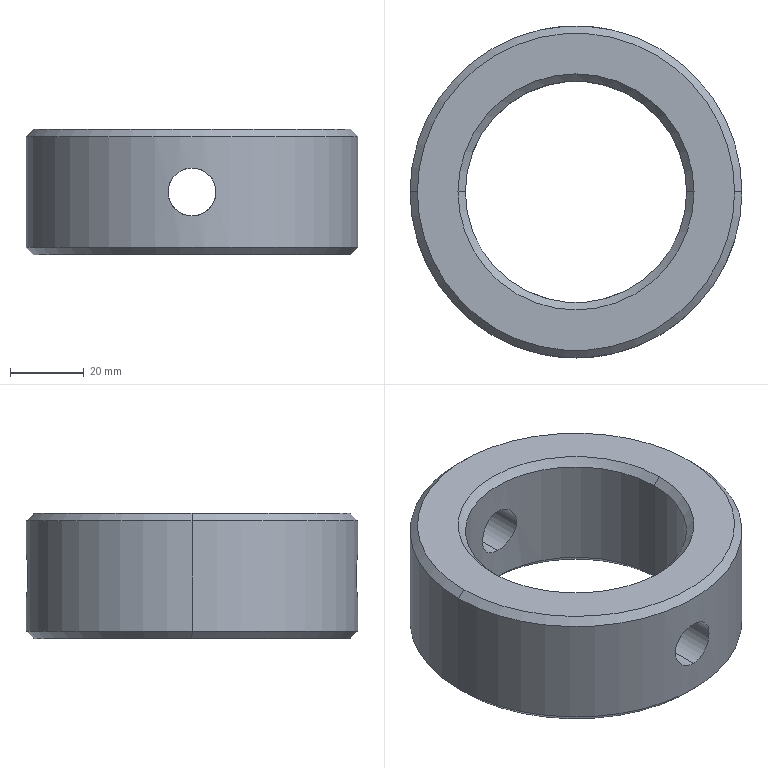Part | SolidWorks | features Chamfer 1, Extrusion 1, ICE 1 | 1 solid | 18 faces | box 90 x 90 x 34 mm | volume 114282 mm3 | cone 8 | cylinder 8 | plane 2 | commonest cylinder face diameters 13 x4 60 x2 90 x2
STEP:
#1=CARTESIAN_POINT('',(43.,0.,34.));
#2=VERTEX_POINT('',#1);
#3=CARTESIAN_POINT('',(-43.,0.,34.));
#4=VERTEX_POINT('',#3);
#5=CARTESIAN_POINT('',(0.,0.,34.));
#6=DIRECTION('',(0.,0.,1.));
#7=DIRECTION('',(1.,0.,0.));
#8=AXIS2_PLACEMENT_3D('',#5,#6,#7);
#9=CIRCLE('',#8,43.);
#10=EDGE_CURVE('',#2,#4,#9,.T.);
#11=ORIENTED_EDGE('',*,*,#10,.F.);
#12=CARTESIAN_POINT('',(45.,0.,32.));
#13=VERTEX_POINT('',#12);
#14=CARTESIAN_POINT('',(43.,0.,34.));
#15=DIRECTION('',(0.7071,0.,-0.7071));
#16=VECTOR('',#15,1000.);
#17=LINE('',#14,#16);
#18=EDGE_CURVE('',#2,#13,#17,.T.);
#19=ORIENTED_EDGE('',*,*,#18,.T.);
#20=CARTESIAN_POINT('',(-45.,0.,32.));
#21=VERTEX_POINT('',#20);
#22=CARTESIAN_POINT('',(0.,0.,32.));
#23=DIRECTION('',(0.,0.,-1.));
#24=DIRECTION('',(1.,0.,0.));
#25=AXIS2_PLACEMENT_3D('',#22,#23,#24);
#26=CIRCLE('',#25,45.);
#27=EDGE_CURVE('',#21,#13,#26,.T.);
#28=ORIENTED_EDGE('',*,*,#27,.F.);
#29=CARTESIAN_POINT('',(-43.,0.,34.));
#30=DIRECTION('',(-0.7071,0.,-0.7071));
#31=VECTOR('',#30,1000.);
#32=LINE('',#29,#31);
#33=EDGE_CURVE('',#4,#21,#32,.T.);
#34=ORIENTED_EDGE('',*,*,#33,.F.);
#35=EDGE_LOOP('',(#11,#19,#28,#34));
#36=FACE_OUTER_BOUND('',#35,.T.);
#37=CARTESIAN_POINT('',(0.,0.,34.));
#38=DIRECTION('',(0.,0.,-1.));
#39=DIRECTION('',(-1.,0.,0.));
#40=AXIS2_PLACEMENT_3D('',#37,#38,#39);
#41=CONICAL_SURFACE('',#40,43.,0.7854);
#42=ADVANCED_FACE('',(#36),#41,.T.);
#43=CARTESIAN_POINT('',(-30.,0.,32.));
#44=VERTEX_POINT('',#43);
#45=CARTESIAN_POINT('',(30.,0.,32.));
#46=VERTEX_POINT('',#45);
#47=CARTESIAN_POINT('',(0.,0.,32.));
#48=DIRECTION('',(0.,0.,1.));
#49=DIRECTION('',(1.,0.,0.));
#50=AXIS2_PLACEMENT_3D('',#47,#48,#49);
#51=CIRCLE('',#50,30.);
#52=EDGE_CURVE('',#44,#46,#51,.T.);
#53=ORIENTED_EDGE('',*,*,#52,.F.);
#54=CARTESIAN_POINT('',(-32.,0.,34.));
#55=VERTEX_POINT('',#54);
#56=CARTESIAN_POINT('',(-30.,0.,32.));
#57=DIRECTION('',(-0.7071,0.,0.7071));
#58=VECTOR('',#57,1000.);
#59=LINE('',#56,#58);
#60=EDGE_CURVE('',#44,#55,#59,.T.);
#61=ORIENTED_EDGE('',*,*,#60,.T.);
#62=CARTESIAN_POINT('',(32.,0.,34.));
#63=VERTEX_POINT('',#62);
#64=CARTESIAN_POINT('',(0.,0.,34.));
#65=DIRECTION('',(0.,0.,-1.));
#66=DIRECTION('',(1.,0.,0.));
#67=AXIS2_PLACEMENT_3D('',#64,#65,#66);
#68=CIRCLE('',#67,32.);
#69=EDGE_CURVE('',#63,#55,#68,.T.);
#70=ORIENTED_EDGE('',*,*,#69,.F.);
#71=CARTESIAN_POINT('',(30.,0.,32.));
#72=DIRECTION('',(0.7071,0.,0.7071));
#73=VECTOR('',#72,1000.);
#74=LINE('',#71,#73);
#75=EDGE_CURVE('',#46,#63,#74,.T.);
#76=ORIENTED_EDGE('',*,*,#75,.F.);
#77=EDGE_LOOP('',(#53,#61,#70,#76));
#78=FACE_OUTER_BOUND('',#77,.T.);
#79=CARTESIAN_POINT('',(0.,0.,32.));
#80=DIRECTION('',(0.,0.,1.));
#81=DIRECTION('',(1.,0.,0.));
#82=AXIS2_PLACEMENT_3D('',#79,#80,#81);
#83=CONICAL_SURFACE('',#82,30.,0.7854);
#84=ADVANCED_FACE('',(#78),#83,.F.);
#85=CARTESIAN_POINT('',(-43.,0.,0.));
#86=VERTEX_POINT('',#85);
#87=CARTESIAN_POINT('',(43.,0.,0.));
#88=VERTEX_POINT('',#87);
#89=CARTESIAN_POINT('',(0.,0.,0.));
#90=DIRECTION('',(0.,0.,-1.));
#91=DIRECTION('',(1.,0.,0.));
#92=AXIS2_PLACEMENT_3D('',#89,#90,#91);
#93=CIRCLE('',#92,43.);
#94=EDGE_CURVE('',#86,#88,#93,.T.);
#95=ORIENTED_EDGE('',*,*,#94,.F.);
#96=CARTESIAN_POINT('',(-45.,0.,2.));
#97=VERTEX_POINT('',#96);
#98=CARTESIAN_POINT('',(-45.,0.,2.));
#99=DIRECTION('',(-0.7071,0.,0.7071));
#100=VECTOR('',#99,1000.);
#101=LINE('',#98,#100);
#102=EDGE_CURVE('',#86,#97,#101,.T.);
#103=ORIENTED_EDGE('',*,*,#102,.T.);
#104=CARTESIAN_POINT('',(45.,0.,2.));
#105=VERTEX_POINT('',#104);
#106=CARTESIAN_POINT('',(0.,0.,2.));
#107=DIRECTION('',(0.,0.,1.));
#108=DIRECTION('',(1.,0.,0.));
#109=AXIS2_PLACEMENT_3D('',#106,#107,#108);
#110=CIRCLE('',#109,45.);
#111=EDGE_CURVE('',#105,#97,#110,.T.);
#112=ORIENTED_EDGE('',*,*,#111,.F.);
#113=CARTESIAN_POINT('',(45.,0.,2.));
#114=DIRECTION('',(0.7071,0.,0.7071));
#115=VECTOR('',#114,1000.);
#116=LINE('',#113,#115);
#117=EDGE_CURVE('',#88,#105,#116,.T.);
#118=ORIENTED_EDGE('',*,*,#117,.F.);
#119=EDGE_LOOP('',(#95,#103,#112,#118));
#120=FACE_OUTER_BOUND('',#119,.T.);
#121=CARTESIAN_POINT('',(0.,0.,2.));
#122=DIRECTION('',(0.,0.,1.));
#123=DIRECTION('',(1.,0.,0.));
#124=AXIS2_PLACEMENT_3D('',#121,#122,#123);
#125=CONICAL_SURFACE('',#124,45.,0.7854);
#126=ADVANCED_FACE('',(#120),#125,.T.);
#127=CARTESIAN_POINT('',(30.,0.,2.));
#128=VERTEX_POINT('',#127);
#129=CARTESIAN_POINT('',(-30.,0.,2.));
#130=VERTEX_POINT('',#129);
#131=CARTESIAN_POINT('',(0.,0.,2.));
#132=DIRECTION('',(0.,0.,-1.));
#133=DIRECTION('',(1.,0.,0.));
#134=AXIS2_PLACEMENT_3D('',#131,#132,#133);
#135=CIRCLE('',#134,30.);
#136=EDGE_CURVE('',#128,#130,#135,.T.);
#137=ORIENTED_EDGE('',*,*,#136,.F.);
#138=CARTESIAN_POINT('',(32.,0.,0.));
#139=VERTEX_POINT('',#138);
#140=CARTESIAN_POINT('',(32.,0.,0.));
#141=DIRECTION('',(0.7071,0.,-0.7071));
#142=VECTOR('',#141,1000.);
#143=LINE('',#140,#142);
#144=EDGE_CURVE('',#128,#139,#143,.T.);
#145=ORIENTED_EDGE('',*,*,#144,.T.);
#146=CARTESIAN_POINT('',(-32.,0.,0.));
#147=VERTEX_POINT('',#146);
#148=CARTESIAN_POINT('',(0.,0.,0.));
#149=DIRECTION('',(0.,0.,1.));
#150=DIRECTION('',(1.,0.,0.));
#151=AXIS2_PLACEMENT_3D('',#148,#149,#150);
#152=CIRCLE('',#151,32.);
#153=EDGE_CURVE('',#147,#139,#152,.T.);
#154=ORIENTED_EDGE('',*,*,#153,.F.);
#155=CARTESIAN_POINT('',(-32.,0.,0.));
#156=DIRECTION('',(-0.7071,0.,-0.7071));
#157=VECTOR('',#156,1000.);
#158=LINE('',#155,#157);
#159=EDGE_CURVE('',#130,#147,#158,.T.);
#160=ORIENTED_EDGE('',*,*,#159,.F.);
#161=EDGE_LOOP('',(#137,#145,#154,#160));
#162=FACE_OUTER_BOUND('',#161,.T.);
#163=CARTESIAN_POINT('',(0.,0.,0.));
#164=DIRECTION('',(0.,0.,-1.));
#165=DIRECTION('',(-1.,0.,0.));
#166=AXIS2_PLACEMENT_3D('',#163,#164,#165);
#167=CONICAL_SURFACE('',#166,32.,0.7854);
#168=ADVANCED_FACE('',(#162),#167,.F.);
#169=CARTESIAN_POINT('',(0.,-45.,10.5));
#170=VERTEX_POINT('',#169);
#171=CARTESIAN_POINT('',(0.,-45.,23.5));
#172=VERTEX_POINT('',#171);
#173=CARTESIAN_POINT('',(0.,-45.,10.5));
#174=CARTESIAN_POINT('',(-0.4244,-45.,10.5));
#175=CARTESIAN_POINT('',(-0.8466,-44.994,10.541));
#176=CARTESIAN_POINT('',(-1.477,-44.976,10.666));
#177=CARTESIAN_POINT('',(-1.685,-44.969,10.719));
#178=CARTESIAN_POINT('',(-2.092,-44.952,10.842));
#179=CARTESIAN_POINT('',(-2.491,-44.932,10.985));
#180=CARTESIAN_POINT('',(-2.875,-44.908,11.166));
#181=CARTESIAN_POINT('',(-3.25,-44.883,11.367));
#182=CARTESIAN_POINT('',(-3.434,-44.869,11.477));
#183=CARTESIAN_POINT('',(-3.967,-44.826,11.833));
#184=CARTESIAN_POINT('',(-4.293,-44.796,12.101));
#185=CARTESIAN_POINT('',(-4.893,-44.734,12.7));
#186=CARTESIAN_POINT('',(-5.167,-44.703,13.034));
#187=CARTESIAN_POINT('',(-5.639,-44.646,13.739));
#188=CARTESIAN_POINT('',(-5.839,-44.62,14.112));
#189=CARTESIAN_POINT('',(-6.084,-44.587,14.702));
#190=CARTESIAN_POINT('',(-6.157,-44.577,14.905));
#191=CARTESIAN_POINT('',(-6.281,-44.56,15.313));
#192=CARTESIAN_POINT('',(-6.333,-44.552,15.519));
#193=CARTESIAN_POINT('',(-6.457,-44.534,16.143));
#194=CARTESIAN_POINT('',(-6.5,-44.528,16.566));
#195=CARTESIAN_POINT('',(-6.5,-44.528,17.425));
#196=CARTESIAN_POINT('',(-6.458,-44.534,17.848));
#197=CARTESIAN_POINT('',(-6.335,-44.552,18.472));
#198=CARTESIAN_POINT('',(-6.283,-44.559,18.678));
#199=CARTESIAN_POINT('',(-6.16,-44.576,19.087));
#200=CARTESIAN_POINT('',(-6.087,-44.586,19.29));
#201=CARTESIAN_POINT('',(-5.843,-44.619,19.88));
#202=CARTESIAN_POINT('',(-5.643,-44.645,20.253));
#203=CARTESIAN_POINT('',(-5.172,-44.702,20.96));
#204=CARTESIAN_POINT('',(-4.898,-44.734,21.294));
#205=CARTESIAN_POINT('',(-4.3,-44.795,21.893));
#206=CARTESIAN_POINT('',(-3.974,-44.826,22.162));
#207=CARTESIAN_POINT('',(-3.263,-44.883,22.638));
#208=CARTESIAN_POINT('',(-2.887,-44.909,22.839));
#209=CARTESIAN_POINT('',(-2.3,-44.942,23.083));
#210=CARTESIAN_POINT('',(-2.101,-44.951,23.155));
#211=CARTESIAN_POINT('',(-1.694,-44.969,23.279));
#212=CARTESIAN_POINT('',(-1.485,-44.976,23.332));
#213=CARTESIAN_POINT('',(-0.8549,-44.994,23.458));
#214=CARTESIAN_POINT('',(-0.43,-45.,23.5));
#215=CARTESIAN_POINT('',(0.,-45.,23.5));
#216=B_SPLINE_CURVE_WITH_KNOTS('',3,(#173,#174,#175,#176,#177,#178,#179,#180,#181,#182,#183,#184,#185,#186,#187,#188,#189,#190,#191,#192,#193,#194,#195,#196,#197,#198,#199,#200,#201,#202,#203,#204,#205,#206,#207,#208,#209,#210,#211,#212,#213,#214,#215),.UNSPECIFIED.,.F.,.F.,(4,2,2,1,2,2,2,2,2,2,2,2,2,2,2,2,2,2,2,2,2,4),(0.02035,0.02162,0.02226,0.02289,0.02353,0.02416,0.02543,0.02671,0.02798,0.02861,0.02925,0.03052,0.03179,0.03243,0.03306,0.03433,0.03561,0.03688,0.03815,0.03878,0.03942,0.04069),.UNSPECIFIED.);
#217=EDGE_CURVE('',#170,#172,#216,.T.);
#218=ORIENTED_EDGE('',*,*,#217,.F.);
#219=CARTESIAN_POINT('',(0.,-30.,10.5));
#220=VERTEX_POINT('',#219);
#221=CARTESIAN_POINT('',(0.,-45.,10.5));
#222=DIRECTION('',(0.,1.,0.));
#223=VECTOR('',#222,1000.);
#224=LINE('',#221,#223);
#225=EDGE_CURVE('',#170,#220,#224,.T.);
#226=ORIENTED_EDGE('',*,*,#225,.T.);
#227=CARTESIAN_POINT('',(0.,-30.,23.5));
#228=VERTEX_POINT('',#227);
#229=CARTESIAN_POINT('',(0.,-30.,10.5));
#230=CARTESIAN_POINT('',(-0.4248,-30.,10.5));
#231=CARTESIAN_POINT('',(-0.848,-29.991,10.541));
#232=CARTESIAN_POINT('',(-1.691,-29.955,10.709));
#233=CARTESIAN_POINT('',(-2.099,-29.929,10.834));
#234=CARTESIAN_POINT('',(-2.686,-29.88,11.077));
#235=CARTESIAN_POINT('',(-2.877,-29.862,11.168));
#236=CARTESIAN_POINT('',(-3.253,-29.824,11.369));
#237=CARTESIAN_POINT('',(-3.438,-29.803,11.479));
#238=CARTESIAN_POINT('',(-3.968,-29.739,11.834));
#239=CARTESIAN_POINT('',(-4.294,-29.693,12.102));
#240=CARTESIAN_POINT('',(-4.894,-29.6,12.701));
#241=CARTESIAN_POINT('',(-5.167,-29.553,13.034));
#242=CARTESIAN_POINT('',(-5.638,-29.466,13.737));
#243=CARTESIAN_POINT('',(-5.838,-29.427,14.11));
#244=CARTESIAN_POINT('',(-6.084,-29.377,14.702));
#245=CARTESIAN_POINT('',(-6.157,-29.362,14.904));
#246=CARTESIAN_POINT('',(-6.281,-29.335,15.312));
#247=CARTESIAN_POINT('',(-6.384,-29.313,15.723));
#248=CARTESIAN_POINT('',(-6.447,-29.299,16.143));
#249=CARTESIAN_POINT('',(-6.489,-29.29,16.567));
#250=CARTESIAN_POINT('',(-6.5,-29.287,16.783));
#251=CARTESIAN_POINT('',(-6.5,-29.287,17.426));
#252=CARTESIAN_POINT('',(-6.458,-29.297,17.849));
#253=CARTESIAN_POINT('',(-6.293,-29.333,18.682));
#254=CARTESIAN_POINT('',(-6.167,-29.36,19.097));
#255=CARTESIAN_POINT('',(-5.842,-29.426,19.882));
#256=CARTESIAN_POINT('',(-5.642,-29.466,20.255));
#257=CARTESIAN_POINT('',(-5.288,-29.531,20.786));
#258=CARTESIAN_POINT('',(-5.16,-29.553,20.959));
#259=CARTESIAN_POINT('',(-4.89,-29.599,21.287));
#260=CARTESIAN_POINT('',(-4.748,-29.622,21.444));
#261=CARTESIAN_POINT('',(-4.301,-29.692,21.892));
#262=CARTESIAN_POINT('',(-3.973,-29.738,22.162));
#263=CARTESIAN_POINT('',(-3.262,-29.824,22.638));
#264=CARTESIAN_POINT('',(-2.889,-29.863,22.838));
#265=CARTESIAN_POINT('',(-2.303,-29.912,23.082));
#266=CARTESIAN_POINT('',(-2.103,-29.927,23.154));
#267=CARTESIAN_POINT('',(-1.694,-29.953,23.279));
#268=CARTESIAN_POINT('',(-1.485,-29.964,23.332));
#269=CARTESIAN_POINT('',(-0.8557,-29.991,23.458));
#270=CARTESIAN_POINT('',(-0.4307,-30.,23.5));
#271=CARTESIAN_POINT('',(0.,-30.,23.5));
#272=B_SPLINE_CURVE_WITH_KNOTS('',3,(#229,#230,#231,#232,#233,#234,#235,#236,#237,#238,#239,#240,#241,#242,#243,#244,#245,#246,#247,#248,#249,#250,#251,#252,#253,#254,#255,#256,#257,#258,#259,#260,#261,#262,#263,#264,#265,#266,#267,#268,#269,#270,#271),.UNSPECIFIED.,.F.,.F.,(4,2,2,2,2,2,2,2,2,1,2,2,2,2,2,2,2,2,2,2,2,4),(0.02038,0.02166,0.02293,0.02357,0.0242,0.02548,0.02675,0.02802,0.02866,0.0293,0.02993,0.03057,0.03184,0.03312,0.03439,0.03503,0.03567,0.03694,0.03821,0.03885,0.03949,0.04076),.UNSPECIFIED.);
#273=EDGE_CURVE('',#220,#228,#272,.T.);
#274=ORIENTED_EDGE('',*,*,#273,.T.);
#275=CARTESIAN_POINT('',(0.,-45.,23.5));
#276=DIRECTION('',(0.,1.,0.));
#277=VECTOR('',#276,1000.);
#278=LINE('',#275,#277);
#279=EDGE_CURVE('',#172,#228,#278,.T.);
#280=ORIENTED_EDGE('',*,*,#279,.F.);
#281=EDGE_LOOP('',(#218,#226,#274,#280));
#282=FACE_OUTER_BOUND('',#281,.T.);
#283=CARTESIAN_POINT('',(0.,-45.,17.));
#284=DIRECTION('',(0.,1.,0.));
#285=DIRECTION('',(0.,0.,1.));
#286=AXIS2_PLACEMENT_3D('',#283,#284,#285);
#287=CYLINDRICAL_SURFACE('',#286,6.5);
#288=ADVANCED_FACE('',(#282),#287,.F.);
#289=CARTESIAN_POINT('',(0.,30.,23.5));
#290=VERTEX_POINT('',#289);
#291=CARTESIAN_POINT('',(0.,30.,10.5));
#292=VERTEX_POINT('',#291);
#293=CARTESIAN_POINT('',(0.,30.,23.5));
#294=CARTESIAN_POINT('',(-0.4308,30.,23.5));
#295=CARTESIAN_POINT('',(-0.8542,29.991,23.458));
#296=CARTESIAN_POINT('',(-1.479,29.964,23.333));
#297=CARTESIAN_POINT('',(-1.685,29.953,23.281));
#298=CARTESIAN_POINT('',(-2.094,29.928,23.157));
#299=CARTESIAN_POINT('',(-2.297,29.913,23.084));
#300=CARTESIAN_POINT('',(-2.887,29.863,22.839));
#301=CARTESIAN_POINT('',(-3.26,29.824,22.639));
#302=CARTESIAN_POINT('',(-3.966,29.739,22.168));
#303=CARTESIAN_POINT('',(-4.299,29.692,21.894));
#304=CARTESIAN_POINT('',(-4.896,29.599,21.296));
#305=CARTESIAN_POINT('',(-5.165,29.553,20.97));
#306=CARTESIAN_POINT('',(-5.64,29.466,20.259));
#307=CARTESIAN_POINT('',(-5.841,29.426,19.883));
#308=CARTESIAN_POINT('',(-6.084,29.377,19.297));
#309=CARTESIAN_POINT('',(-6.156,29.362,19.097));
#310=CARTESIAN_POINT('',(-6.28,29.335,18.69));
#311=CARTESIAN_POINT('',(-6.333,29.324,18.48));
#312=CARTESIAN_POINT('',(-6.458,29.297,17.851));
#313=CARTESIAN_POINT('',(-6.5,29.287,17.428));
#314=CARTESIAN_POINT('',(-6.5,29.287,16.577));
#315=CARTESIAN_POINT('',(-6.458,29.297,16.145));
#316=CARTESIAN_POINT('',(-6.291,29.333,15.31));
#317=CARTESIAN_POINT('',(-6.168,29.36,14.905));
#318=CARTESIAN_POINT('',(-5.923,29.41,14.313));
#319=CARTESIAN_POINT('',(-5.83,29.428,14.118));
#320=CARTESIAN_POINT('',(-5.629,29.467,13.743));
#321=CARTESIAN_POINT('',(-5.52,29.488,13.562));
#322=CARTESIAN_POINT('',(-5.168,29.553,13.035));
#323=CARTESIAN_POINT('',(-4.897,29.599,12.705));
#324=CARTESIAN_POINT('',(-4.294,29.693,12.101));
#325=CARTESIAN_POINT('',(-3.967,29.739,11.834));
#326=CARTESIAN_POINT('',(-3.44,29.803,11.481));
#327=CARTESIAN_POINT('',(-3.258,29.823,11.371));
#328=CARTESIAN_POINT('',(-2.881,29.862,11.169));
#329=CARTESIAN_POINT('',(-2.687,29.88,11.077));
#330=CARTESIAN_POINT('',(-2.098,29.929,10.833));
#331=CARTESIAN_POINT('',(-1.692,29.955,10.71));
#332=CARTESIAN_POINT('',(-1.065,29.982,10.584));
#333=CARTESIAN_POINT('',(-0.852,29.989,10.553));
#334=CARTESIAN_POINT('',(-0.4254,29.998,10.51));
#335=CARTESIAN_POINT('',(-0.2125,30.,10.5));
#336=CARTESIAN_POINT('',(0.,30.,10.5));
#337=B_SPLINE_CURVE_WITH_KNOTS('',3,(#293,#294,#295,#296,#297,#298,#299,#300,#301,#302,#303,#304,#305,#306,#307,#308,#309,#310,#311,#312,#313,#314,#315,#316,#317,#318,#319,#320,#321,#322,#323,#324,#325,#326,#327,#328,#329,#330,#331,#332,#333,#334,#335,#336),.UNSPECIFIED.,.F.,.F.,(4,2,2,2,2,2,2,2,2,2,2,2,2,2,2,2,2,2,2,2,2,4),(0.,0.001274,0.001911,0.002548,0.003822,0.005096,0.00637,0.007643,0.00828,0.008917,0.01019,0.01147,0.01274,0.01338,0.01401,0.01529,0.01656,0.0172,0.01783,0.01911,0.01975,0.02038),.UNSPECIFIED.);
#338=EDGE_CURVE('',#290,#292,#337,.T.);
#339=ORIENTED_EDGE('',*,*,#338,.T.);
#340=CARTESIAN_POINT('',(0.,45.,10.5));
#341=VERTEX_POINT('',#340);
#342=CARTESIAN_POINT('',(0.,-45.,10.5));
#343=DIRECTION('',(0.,1.,0.));
#344=VECTOR('',#343,1000.);
#345=LINE('',#342,#344);
#346=EDGE_CURVE('',#292,#341,#345,.T.);
#347=ORIENTED_EDGE('',*,*,#346,.T.);
#348=CARTESIAN_POINT('',(0.,45.,23.5));
#349=VERTEX_POINT('',#348);
#350=CARTESIAN_POINT('',(0.,45.,23.5));
#351=CARTESIAN_POINT('',(-0.4301,45.,23.5));
#352=CARTESIAN_POINT('',(-0.8529,44.994,23.458));
#353=CARTESIAN_POINT('',(-1.477,44.976,23.334));
#354=CARTESIAN_POINT('',(-1.683,44.969,23.282));
#355=CARTESIAN_POINT('',(-2.091,44.952,23.158));
#356=CARTESIAN_POINT('',(-2.294,44.942,23.085));
#357=CARTESIAN_POINT('',(-2.885,44.909,22.84));
#358=CARTESIAN_POINT('',(-3.258,44.883,22.641));
#359=CARTESIAN_POINT('',(-3.964,44.826,22.169));
#360=CARTESIAN_POINT('',(-4.298,44.795,21.895));
#361=CARTESIAN_POINT('',(-4.897,44.734,21.296));
#362=CARTESIAN_POINT('',(-5.165,44.703,20.969));
#363=CARTESIAN_POINT('',(-5.522,44.66,20.436));
#364=CARTESIAN_POINT('',(-5.632,44.646,20.252));
#365=CARTESIAN_POINT('',(-5.833,44.621,19.877));
#366=CARTESIAN_POINT('',(-6.014,44.597,19.494));
#367=CARTESIAN_POINT('',(-6.157,44.577,19.095));
#368=CARTESIAN_POINT('',(-6.281,44.56,18.688));
#369=CARTESIAN_POINT('',(-6.333,44.552,18.479));
#370=CARTESIAN_POINT('',(-6.458,44.534,17.849));
#371=CARTESIAN_POINT('',(-6.5,44.528,17.427));
#372=CARTESIAN_POINT('',(-6.5,44.528,16.578));
#373=CARTESIAN_POINT('',(-6.458,44.534,16.147));
#374=CARTESIAN_POINT('',(-6.291,44.558,15.312));
#375=CARTESIAN_POINT('',(-6.169,44.576,14.907));
#376=CARTESIAN_POINT('',(-5.924,44.608,14.316));
#377=CARTESIAN_POINT('',(-5.832,44.621,14.121));
#378=CARTESIAN_POINT('',(-5.631,44.646,13.745));
#379=CARTESIAN_POINT('',(-5.521,44.66,13.564));
#380=CARTESIAN_POINT('',(-5.169,44.703,13.036));
#381=CARTESIAN_POINT('',(-4.899,44.734,12.707));
#382=CARTESIAN_POINT('',(-4.294,44.796,12.101));
#383=CARTESIAN_POINT('',(-3.966,44.826,11.833));
#384=CARTESIAN_POINT('',(-3.438,44.869,11.48));
#385=CARTESIAN_POINT('',(-3.256,44.882,11.37));
#386=CARTESIAN_POINT('',(-2.88,44.908,11.169));
#387=CARTESIAN_POINT('',(-2.685,44.92,11.077));
#388=CARTESIAN_POINT('',(-2.095,44.953,10.832));
#389=CARTESIAN_POINT('',(-1.69,44.97,10.709));
#390=CARTESIAN_POINT('',(-0.8557,44.994,10.543));
#391=CARTESIAN_POINT('',(-0.4245,45.,10.5));
#392=CARTESIAN_POINT('',(0.,45.,10.5));
#393=B_SPLINE_CURVE_WITH_KNOTS('',3,(#350,#351,#352,#353,#354,#355,#356,#357,#358,#359,#360,#361,#362,#363,#364,#365,#366,#367,#368,#369,#370,#371,#372,#373,#374,#375,#376,#377,#378,#379,#380,#381,#382,#383,#384,#385,#386,#387,#388,#389,#390,#391,#392),.UNSPECIFIED.,.F.,.F.,(4,2,2,2,2,2,2,2,1,2,2,2,2,2,2,2,2,2,2,2,2,4),(0.,0.001272,0.001908,0.002544,0.003815,0.005087,0.006359,0.006995,0.007631,0.008267,0.008903,0.01017,0.01145,0.01272,0.01335,0.01399,0.01526,0.01653,0.01717,0.01781,0.01908,0.02035),.UNSPECIFIED.);
#394=EDGE_CURVE('',#349,#341,#393,.T.);
#395=ORIENTED_EDGE('',*,*,#394,.F.);
#396=CARTESIAN_POINT('',(0.,-45.,23.5));
#397=DIRECTION('',(0.,1.,0.));
#398=VECTOR('',#397,1000.);
#399=LINE('',#396,#398);
#400=EDGE_CURVE('',#290,#349,#399,.T.);
#401=ORIENTED_EDGE('',*,*,#400,.F.);
#402=EDGE_LOOP('',(#339,#347,#395,#401));
#403=FACE_OUTER_BOUND('',#402,.T.);
#404=CARTESIAN_POINT('',(0.,-45.,17.));
#405=DIRECTION('',(0.,1.,0.));
#406=DIRECTION('',(0.,0.,1.));
#407=AXIS2_PLACEMENT_3D('',#404,#405,#406);
#408=CYLINDRICAL_SURFACE('',#407,6.5);
#409=ADVANCED_FACE('',(#403),#408,.F.);
#410=CARTESIAN_POINT('',(0.,-30.,23.5));
#411=CARTESIAN_POINT('',(0.4308,-30.,23.5));
#412=CARTESIAN_POINT('',(0.8542,-29.991,23.458));
#413=CARTESIAN_POINT('',(1.479,-29.964,23.333));
#414=CARTESIAN_POINT('',(1.685,-29.953,23.281));
#415=CARTESIAN_POINT('',(2.094,-29.928,23.157));
#416=CARTESIAN_POINT('',(2.297,-29.913,23.084));
#417=CARTESIAN_POINT('',(2.887,-29.863,22.839));
#418=CARTESIAN_POINT('',(3.26,-29.824,22.639));
#419=CARTESIAN_POINT('',(3.966,-29.739,22.168));
#420=CARTESIAN_POINT('',(4.299,-29.692,21.894));
#421=CARTESIAN_POINT('',(4.896,-29.599,21.296));
#422=CARTESIAN_POINT('',(5.165,-29.553,20.97));
#423=CARTESIAN_POINT('',(5.64,-29.466,20.259));
#424=CARTESIAN_POINT('',(5.841,-29.426,19.883));
#425=CARTESIAN_POINT('',(6.084,-29.377,19.297));
#426=CARTESIAN_POINT('',(6.156,-29.362,19.097));
#427=CARTESIAN_POINT('',(6.28,-29.335,18.69));
#428=CARTESIAN_POINT('',(6.333,-29.324,18.48));
#429=CARTESIAN_POINT('',(6.458,-29.297,17.851));
#430=CARTESIAN_POINT('',(6.5,-29.287,17.428));
#431=CARTESIAN_POINT('',(6.5,-29.287,16.577));
#432=CARTESIAN_POINT('',(6.458,-29.297,16.145));
#433=CARTESIAN_POINT('',(6.291,-29.333,15.31));
#434=CARTESIAN_POINT('',(6.168,-29.36,14.905));
#435=CARTESIAN_POINT('',(5.923,-29.41,14.313));
#436=CARTESIAN_POINT('',(5.83,-29.428,14.118));
#437=CARTESIAN_POINT('',(5.629,-29.467,13.743));
#438=CARTESIAN_POINT('',(5.52,-29.488,13.562));
#439=CARTESIAN_POINT('',(5.168,-29.553,13.035));
#440=CARTESIAN_POINT('',(4.897,-29.599,12.705));
#441=CARTESIAN_POINT('',(4.294,-29.693,12.101));
#442=CARTESIAN_POINT('',(3.967,-29.739,11.834));
#443=CARTESIAN_POINT('',(3.44,-29.803,11.481));
#444=CARTESIAN_POINT('',(3.258,-29.823,11.371));
#445=CARTESIAN_POINT('',(2.881,-29.862,11.169));
#446=CARTESIAN_POINT('',(2.687,-29.88,11.077));
#447=CARTESIAN_POINT('',(2.098,-29.929,10.833));
#448=CARTESIAN_POINT('',(1.692,-29.955,10.71));
#449=CARTESIAN_POINT('',(1.065,-29.982,10.584));
#450=CARTESIAN_POINT('',(0.852,-29.989,10.553));
#451=CARTESIAN_POINT('',(0.4254,-29.998,10.51));
#452=CARTESIAN_POINT('',(0.2125,-30.,10.5));
#453=CARTESIAN_POINT('',(0.,-30.,10.5));
#454=B_SPLINE_CURVE_WITH_KNOTS('',3,(#410,#411,#412,#413,#414,#415,#416,#417,#418,#419,#420,#421,#422,#423,#424,#425,#426,#427,#428,#429,#430,#431,#432,#433,#434,#435,#436,#437,#438,#439,#440,#441,#442,#443,#444,#445,#446,#447,#448,#449,#450,#451,#452,#453),.UNSPECIFIED.,.F.,.F.,(4,2,2,2,2,2,2,2,2,2,2,2,2,2,2,2,2,2,2,2,2,4),(0.,0.001274,0.001911,0.002548,0.003822,0.005096,0.00637,0.007643,0.00828,0.008917,0.01019,0.01147,0.01274,0.01338,0.01401,0.01529,0.01656,0.0172,0.01783,0.01911,0.01975,0.02038),.UNSPECIFIED.);
#455=EDGE_CURVE('',#228,#220,#454,.T.);
#456=ORIENTED_EDGE('',*,*,#455,.F.);
#457=ORIENTED_EDGE('',*,*,#273,.F.);
#458=EDGE_LOOP('',(#456,#457));
#459=FACE_BOUND('',#458,.T.);
#460=ORIENTED_EDGE('',*,*,#52,.T.);
#461=CARTESIAN_POINT('',(30.,0.,34.));
#462=DIRECTION('',(0.,0.,-1.));
#463=VECTOR('',#462,1000.);
#464=LINE('',#461,#463);
#465=EDGE_CURVE('',#46,#128,#464,.T.);
#466=ORIENTED_EDGE('',*,*,#465,.T.);
#467=ORIENTED_EDGE('',*,*,#136,.T.);
#468=CARTESIAN_POINT('',(-30.,0.,34.));
#469=DIRECTION('',(0.,0.,-1.));
#470=VECTOR('',#469,1000.);
#471=LINE('',#468,#470);
#472=EDGE_CURVE('',#44,#130,#471,.T.);
#473=ORIENTED_EDGE('',*,*,#472,.F.);
#474=EDGE_LOOP('',(#460,#466,#467,#473));
#475=FACE_OUTER_BOUND('',#474,.T.);
#476=CARTESIAN_POINT('',(0.,0.,34.));
#477=DIRECTION('',(0.,0.,-1.));
#478=DIRECTION('',(-1.,0.,0.));
#479=AXIS2_PLACEMENT_3D('',#476,#477,#478);
#480=CYLINDRICAL_SURFACE('',#479,30.);
#481=ADVANCED_FACE('',(#459,#475),#480,.F.);
#482=ORIENTED_EDGE('',*,*,#394,.T.);
#483=CARTESIAN_POINT('',(0.,45.,10.5));
#484=CARTESIAN_POINT('',(0.4244,45.,10.5));
#485=CARTESIAN_POINT('',(0.8466,44.994,10.541));
#486=CARTESIAN_POINT('',(1.477,44.976,10.666));
#487=CARTESIAN_POINT('',(1.685,44.969,10.719));
#488=CARTESIAN_POINT('',(2.092,44.952,10.842));
#489=CARTESIAN_POINT('',(2.491,44.932,10.985));
#490=CARTESIAN_POINT('',(2.875,44.908,11.166));
#491=CARTESIAN_POINT('',(3.25,44.883,11.367));
#492=CARTESIAN_POINT('',(3.434,44.869,11.477));
#493=CARTESIAN_POINT('',(3.967,44.826,11.833));
#494=CARTESIAN_POINT('',(4.293,44.796,12.101));
#495=CARTESIAN_POINT('',(4.893,44.734,12.7));
#496=CARTESIAN_POINT('',(5.167,44.703,13.034));
#497=CARTESIAN_POINT('',(5.639,44.646,13.739));
#498=CARTESIAN_POINT('',(5.839,44.62,14.112));
#499=CARTESIAN_POINT('',(6.084,44.587,14.702));
#500=CARTESIAN_POINT('',(6.157,44.577,14.905));
#501=CARTESIAN_POINT('',(6.281,44.56,15.313));
#502=CARTESIAN_POINT('',(6.333,44.552,15.519));
#503=CARTESIAN_POINT('',(6.457,44.534,16.143));
#504=CARTESIAN_POINT('',(6.5,44.528,16.566));
#505=CARTESIAN_POINT('',(6.5,44.528,17.425));
#506=CARTESIAN_POINT('',(6.458,44.534,17.848));
#507=CARTESIAN_POINT('',(6.335,44.552,18.472));
#508=CARTESIAN_POINT('',(6.283,44.559,18.678));
#509=CARTESIAN_POINT('',(6.16,44.576,19.087));
#510=CARTESIAN_POINT('',(6.087,44.586,19.29));
#511=CARTESIAN_POINT('',(5.843,44.619,19.88));
#512=CARTESIAN_POINT('',(5.643,44.645,20.253));
#513=CARTESIAN_POINT('',(5.172,44.702,20.96));
#514=CARTESIAN_POINT('',(4.898,44.734,21.294));
#515=CARTESIAN_POINT('',(4.3,44.795,21.893));
#516=CARTESIAN_POINT('',(3.974,44.826,22.162));
#517=CARTESIAN_POINT('',(3.263,44.883,22.638));
#518=CARTESIAN_POINT('',(2.887,44.909,22.839));
#519=CARTESIAN_POINT('',(2.3,44.942,23.083));
#520=CARTESIAN_POINT('',(2.101,44.951,23.155));
#521=CARTESIAN_POINT('',(1.694,44.969,23.279));
#522=CARTESIAN_POINT('',(1.485,44.976,23.332));
#523=CARTESIAN_POINT('',(0.8549,44.994,23.458));
#524=CARTESIAN_POINT('',(0.43,45.,23.5));
#525=CARTESIAN_POINT('',(0.,45.,23.5));
#526=B_SPLINE_CURVE_WITH_KNOTS('',3,(#483,#484,#485,#486,#487,#488,#489,#490,#491,#492,#493,#494,#495,#496,#497,#498,#499,#500,#501,#502,#503,#504,#505,#506,#507,#508,#509,#510,#511,#512,#513,#514,#515,#516,#517,#518,#519,#520,#521,#522,#523,#524,#525),.UNSPECIFIED.,.F.,.F.,(4,2,2,1,2,2,2,2,2,2,2,2,2,2,2,2,2,2,2,2,2,4),(0.02035,0.02162,0.02226,0.02289,0.02353,0.02416,0.02543,0.02671,0.02798,0.02861,0.02925,0.03052,0.03179,0.03243,0.03306,0.03433,0.03561,0.03688,0.03815,0.03878,0.03942,0.04069),.UNSPECIFIED.);
#527=EDGE_CURVE('',#341,#349,#526,.T.);
#528=ORIENTED_EDGE('',*,*,#527,.T.);
#529=EDGE_LOOP('',(#482,#528));
#530=FACE_BOUND('',#529,.T.);
#531=ORIENTED_EDGE('',*,*,#27,.T.);
#532=CARTESIAN_POINT('',(45.,0.,34.));
#533=DIRECTION('',(0.,0.,-1.));
#534=VECTOR('',#533,1000.);
#535=LINE('',#532,#534);
#536=EDGE_CURVE('',#13,#105,#535,.T.);
#537=ORIENTED_EDGE('',*,*,#536,.T.);
#538=ORIENTED_EDGE('',*,*,#111,.T.);
#539=CARTESIAN_POINT('',(-45.,0.,34.));
#540=DIRECTION('',(0.,0.,-1.));
#541=VECTOR('',#540,1000.);
#542=LINE('',#539,#541);
#543=EDGE_CURVE('',#21,#97,#542,.T.);
#544=ORIENTED_EDGE('',*,*,#543,.F.);
#545=EDGE_LOOP('',(#531,#537,#538,#544));
#546=FACE_OUTER_BOUND('',#545,.T.);
#547=CARTESIAN_POINT('',(0.,0.,34.));
#548=DIRECTION('',(0.,0.,-1.));
#549=DIRECTION('',(-1.,0.,0.));
#550=AXIS2_PLACEMENT_3D('',#547,#548,#549);
#551=CYLINDRICAL_SURFACE('',#550,45.);
#552=ADVANCED_FACE('',(#530,#546),#551,.T.);
#553=ORIENTED_EDGE('',*,*,#69,.T.);
#554=CARTESIAN_POINT('',(0.,0.,34.));
#555=DIRECTION('',(0.,0.,-1.));
#556=DIRECTION('',(1.,0.,0.));
#557=AXIS2_PLACEMENT_3D('',#554,#555,#556);
#558=CIRCLE('',#557,32.);
#559=EDGE_CURVE('',#55,#63,#558,.T.);
#560=ORIENTED_EDGE('',*,*,#559,.T.);
#561=EDGE_LOOP('',(#553,#560));
#562=FACE_BOUND('',#561,.T.);
#563=CARTESIAN_POINT('',(0.,0.,34.));
#564=DIRECTION('',(0.,0.,1.));
#565=DIRECTION('',(1.,0.,0.));
#566=AXIS2_PLACEMENT_3D('',#563,#564,#565);
#567=CIRCLE('',#566,43.);
#568=EDGE_CURVE('',#4,#2,#567,.T.);
#569=ORIENTED_EDGE('',*,*,#568,.T.);
#570=ORIENTED_EDGE('',*,*,#10,.T.);
#571=EDGE_LOOP('',(#569,#570));
#572=FACE_OUTER_BOUND('',#571,.T.);
#573=CARTESIAN_POINT('',(0.,0.,34.));
#574=DIRECTION('',(0.,0.,1.));
#575=DIRECTION('',(1.,0.,0.));
#576=AXIS2_PLACEMENT_3D('',#573,#574,#575);
#577=PLANE('',#576);
#578=ADVANCED_FACE('',(#562,#572),#577,.T.);
#579=ORIENTED_EDGE('',*,*,#153,.T.);
#580=CARTESIAN_POINT('',(0.,0.,0.));
#581=DIRECTION('',(0.,0.,1.));
#582=DIRECTION('',(1.,0.,0.));
#583=AXIS2_PLACEMENT_3D('',#580,#581,#582);
#584=CIRCLE('',#583,32.);
#585=EDGE_CURVE('',#139,#147,#584,.T.);
#586=ORIENTED_EDGE('',*,*,#585,.T.);
#587=EDGE_LOOP('',(#579,#586));
#588=FACE_BOUND('',#587,.T.);
#589=CARTESIAN_POINT('',(0.,0.,0.));
#590=DIRECTION('',(0.,0.,-1.));
#591=DIRECTION('',(1.,0.,0.));
#592=AXIS2_PLACEMENT_3D('',#589,#590,#591);
#593=CIRCLE('',#592,43.);
#594=EDGE_CURVE('',#88,#86,#593,.T.);
#595=ORIENTED_EDGE('',*,*,#594,.T.);
#596=ORIENTED_EDGE('',*,*,#94,.T.);
#597=EDGE_LOOP('',(#595,#596));
#598=FACE_OUTER_BOUND('',#597,.T.);
#599=CARTESIAN_POINT('',(0.,0.,0.));
#600=DIRECTION('',(0.,0.,1.));
#601=DIRECTION('',(1.,0.,0.));
#602=AXIS2_PLACEMENT_3D('',#599,#600,#601);
#603=PLANE('',#602);
#604=ADVANCED_FACE('',(#588,#598),#603,.F.);
#605=ORIENTED_EDGE('',*,*,#536,.F.);
#606=CARTESIAN_POINT('',(0.,0.,32.));
#607=DIRECTION('',(0.,0.,-1.));
#608=DIRECTION('',(1.,0.,0.));
#609=AXIS2_PLACEMENT_3D('',#606,#607,#608);
#610=CIRCLE('',#609,45.);
#611=EDGE_CURVE('',#13,#21,#610,.T.);
#612=ORIENTED_EDGE('',*,*,#611,.T.);
#613=ORIENTED_EDGE('',*,*,#543,.T.);
#614=CARTESIAN_POINT('',(0.,0.,2.));
#615=DIRECTION('',(0.,0.,1.));
#616=DIRECTION('',(1.,0.,0.));
#617=AXIS2_PLACEMENT_3D('',#614,#615,#616);
#618=CIRCLE('',#617,45.);
#619=EDGE_CURVE('',#97,#105,#618,.T.);
#620=ORIENTED_EDGE('',*,*,#619,.T.);
#621=EDGE_LOOP('',(#605,#612,#613,#620));
#622=FACE_OUTER_BOUND('',#621,.T.);
#623=CARTESIAN_POINT('',(0.,-45.,23.5));
#624=CARTESIAN_POINT('',(0.4301,-45.,23.5));
#625=CARTESIAN_POINT('',(0.8529,-44.994,23.458));
#626=CARTESIAN_POINT('',(1.477,-44.976,23.334));
#627=CARTESIAN_POINT('',(1.683,-44.969,23.282));
#628=CARTESIAN_POINT('',(2.091,-44.952,23.158));
#629=CARTESIAN_POINT('',(2.294,-44.942,23.085));
#630=CARTESIAN_POINT('',(2.885,-44.909,22.84));
#631=CARTESIAN_POINT('',(3.258,-44.883,22.641));
#632=CARTESIAN_POINT('',(3.964,-44.826,22.169));
#633=CARTESIAN_POINT('',(4.298,-44.795,21.895));
#634=CARTESIAN_POINT('',(4.897,-44.734,21.296));
#635=CARTESIAN_POINT('',(5.165,-44.703,20.969));
#636=CARTESIAN_POINT('',(5.522,-44.66,20.436));
#637=CARTESIAN_POINT('',(5.632,-44.646,20.252));
#638=CARTESIAN_POINT('',(5.833,-44.621,19.877));
#639=CARTESIAN_POINT('',(6.014,-44.597,19.494));
#640=CARTESIAN_POINT('',(6.157,-44.577,19.095));
#641=CARTESIAN_POINT('',(6.281,-44.56,18.688));
#642=CARTESIAN_POINT('',(6.333,-44.552,18.479));
#643=CARTESIAN_POINT('',(6.458,-44.534,17.849));
#644=CARTESIAN_POINT('',(6.5,-44.528,17.427));
#645=CARTESIAN_POINT('',(6.5,-44.528,16.578));
#646=CARTESIAN_POINT('',(6.458,-44.534,16.147));
#647=CARTESIAN_POINT('',(6.291,-44.558,15.312));
#648=CARTESIAN_POINT('',(6.169,-44.576,14.907));
#649=CARTESIAN_POINT('',(5.924,-44.608,14.316));
#650=CARTESIAN_POINT('',(5.832,-44.621,14.121));
#651=CARTESIAN_POINT('',(5.631,-44.646,13.745));
#652=CARTESIAN_POINT('',(5.521,-44.66,13.564));
#653=CARTESIAN_POINT('',(5.169,-44.703,13.036));
#654=CARTESIAN_POINT('',(4.899,-44.734,12.707));
#655=CARTESIAN_POINT('',(4.294,-44.796,12.101));
#656=CARTESIAN_POINT('',(3.966,-44.826,11.833));
#657=CARTESIAN_POINT('',(3.438,-44.869,11.48));
#658=CARTESIAN_POINT('',(3.256,-44.882,11.37));
#659=CARTESIAN_POINT('',(2.88,-44.908,11.169));
#660=CARTESIAN_POINT('',(2.685,-44.92,11.077));
#661=CARTESIAN_POINT('',(2.095,-44.953,10.832));
#662=CARTESIAN_POINT('',(1.69,-44.97,10.709));
#663=CARTESIAN_POINT('',(0.8557,-44.994,10.543));
#664=CARTESIAN_POINT('',(0.4245,-45.,10.5));
#665=CARTESIAN_POINT('',(0.,-45.,10.5));
#666=B_SPLINE_CURVE_WITH_KNOTS('',3,(#623,#624,#625,#626,#627,#628,#629,#630,#631,#632,#633,#634,#635,#636,#637,#638,#639,#640,#641,#642,#643,#644,#645,#646,#647,#648,#649,#650,#651,#652,#653,#654,#655,#656,#657,#658,#659,#660,#661,#662,#663,#664,#665),.UNSPECIFIED.,.F.,.F.,(4,2,2,2,2,2,2,2,1,2,2,2,2,2,2,2,2,2,2,2,2,4),(0.,0.001272,0.001908,0.002544,0.003815,0.005087,0.006359,0.006995,0.007631,0.008267,0.008903,0.01017,0.01145,0.01272,0.01335,0.01399,0.01526,0.01653,0.01717,0.01781,0.01908,0.02035),.UNSPECIFIED.);
#667=EDGE_CURVE('',#172,#170,#666,.T.);
#668=ORIENTED_EDGE('',*,*,#667,.T.);
#669=ORIENTED_EDGE('',*,*,#217,.T.);
#670=EDGE_LOOP('',(#668,#669));
#671=FACE_BOUND('',#670,.T.);
#672=CARTESIAN_POINT('',(0.,0.,34.));
#673=DIRECTION('',(0.,0.,-1.));
#674=DIRECTION('',(-1.,0.,0.));
#675=AXIS2_PLACEMENT_3D('',#672,#673,#674);
#676=CYLINDRICAL_SURFACE('',#675,45.);
#677=ADVANCED_FACE('',(#622,#671),#676,.T.);
#678=ORIENTED_EDGE('',*,*,#465,.F.);
#679=CARTESIAN_POINT('',(0.,0.,32.));
#680=DIRECTION('',(0.,0.,1.));
#681=DIRECTION('',(1.,0.,0.));
#682=AXIS2_PLACEMENT_3D('',#679,#680,#681);
#683=CIRCLE('',#682,30.);
#684=EDGE_CURVE('',#46,#44,#683,.T.);
#685=ORIENTED_EDGE('',*,*,#684,.T.);
#686=ORIENTED_EDGE('',*,*,#472,.T.);
#687=CARTESIAN_POINT('',(0.,0.,2.));
#688=DIRECTION('',(0.,0.,-1.));
#689=DIRECTION('',(1.,0.,0.));
#690=AXIS2_PLACEMENT_3D('',#687,#688,#689);
#691=CIRCLE('',#690,30.);
#692=EDGE_CURVE('',#130,#128,#691,.T.);
#693=ORIENTED_EDGE('',*,*,#692,.T.);
#694=EDGE_LOOP('',(#678,#685,#686,#693));
#695=FACE_OUTER_BOUND('',#694,.T.);
#696=ORIENTED_EDGE('',*,*,#338,.F.);
#697=CARTESIAN_POINT('',(0.,30.,10.5));
#698=CARTESIAN_POINT('',(0.4248,30.,10.5));
#699=CARTESIAN_POINT('',(0.848,29.991,10.541));
#700=CARTESIAN_POINT('',(1.691,29.955,10.709));
#701=CARTESIAN_POINT('',(2.099,29.929,10.834));
#702=CARTESIAN_POINT('',(2.686,29.88,11.077));
#703=CARTESIAN_POINT('',(2.877,29.862,11.168));
#704=CARTESIAN_POINT('',(3.253,29.824,11.369));
#705=CARTESIAN_POINT('',(3.438,29.803,11.479));
#706=CARTESIAN_POINT('',(3.968,29.739,11.834));
#707=CARTESIAN_POINT('',(4.294,29.693,12.102));
#708=CARTESIAN_POINT('',(4.894,29.6,12.701));
#709=CARTESIAN_POINT('',(5.167,29.553,13.034));
#710=CARTESIAN_POINT('',(5.638,29.466,13.737));
#711=CARTESIAN_POINT('',(5.838,29.427,14.11));
#712=CARTESIAN_POINT('',(6.084,29.377,14.702));
#713=CARTESIAN_POINT('',(6.157,29.362,14.904));
#714=CARTESIAN_POINT('',(6.281,29.335,15.312));
#715=CARTESIAN_POINT('',(6.384,29.313,15.723));
#716=CARTESIAN_POINT('',(6.447,29.299,16.143));
#717=CARTESIAN_POINT('',(6.489,29.29,16.567));
#718=CARTESIAN_POINT('',(6.5,29.287,16.783));
#719=CARTESIAN_POINT('',(6.5,29.287,17.426));
#720=CARTESIAN_POINT('',(6.458,29.297,17.849));
#721=CARTESIAN_POINT('',(6.293,29.333,18.682));
#722=CARTESIAN_POINT('',(6.167,29.36,19.097));
#723=CARTESIAN_POINT('',(5.842,29.426,19.882));
#724=CARTESIAN_POINT('',(5.642,29.466,20.255));
#725=CARTESIAN_POINT('',(5.288,29.531,20.786));
#726=CARTESIAN_POINT('',(5.16,29.553,20.959));
#727=CARTESIAN_POINT('',(4.89,29.599,21.287));
#728=CARTESIAN_POINT('',(4.748,29.622,21.444));
#729=CARTESIAN_POINT('',(4.301,29.692,21.892));
#730=CARTESIAN_POINT('',(3.973,29.738,22.162));
#731=CARTESIAN_POINT('',(3.262,29.824,22.638));
#732=CARTESIAN_POINT('',(2.889,29.863,22.838));
#733=CARTESIAN_POINT('',(2.303,29.912,23.082));
#734=CARTESIAN_POINT('',(2.103,29.927,23.154));
#735=CARTESIAN_POINT('',(1.694,29.953,23.279));
#736=CARTESIAN_POINT('',(1.485,29.964,23.332));
#737=CARTESIAN_POINT('',(0.8557,29.991,23.458));
#738=CARTESIAN_POINT('',(0.4307,30.,23.5));
#739=CARTESIAN_POINT('',(0.,30.,23.5));
#740=B_SPLINE_CURVE_WITH_KNOTS('',3,(#697,#698,#699,#700,#701,#702,#703,#704,#705,#706,#707,#708,#709,#710,#711,#712,#713,#714,#715,#716,#717,#718,#719,#720,#721,#722,#723,#724,#725,#726,#727,#728,#729,#730,#731,#732,#733,#734,#735,#736,#737,#738,#739),.UNSPECIFIED.,.F.,.F.,(4,2,2,2,2,2,2,2,2,1,2,2,2,2,2,2,2,2,2,2,2,4),(0.02038,0.02166,0.02293,0.02357,0.0242,0.02548,0.02675,0.02802,0.02866,0.0293,0.02993,0.03057,0.03184,0.03312,0.03439,0.03503,0.03567,0.03694,0.03821,0.03885,0.03949,0.04076),.UNSPECIFIED.);
#741=EDGE_CURVE('',#292,#290,#740,.T.);
#742=ORIENTED_EDGE('',*,*,#741,.F.);
#743=EDGE_LOOP('',(#696,#742));
#744=FACE_BOUND('',#743,.T.);
#745=CARTESIAN_POINT('',(0.,0.,34.));
#746=DIRECTION('',(0.,0.,-1.));
#747=DIRECTION('',(-1.,0.,0.));
#748=AXIS2_PLACEMENT_3D('',#745,#746,#747);
#749=CYLINDRICAL_SURFACE('',#748,30.);
#750=ADVANCED_FACE('',(#695,#744),#749,.F.);
#751=ORIENTED_EDGE('',*,*,#346,.F.);
#752=ORIENTED_EDGE('',*,*,#741,.T.);
#753=ORIENTED_EDGE('',*,*,#400,.T.);
#754=ORIENTED_EDGE('',*,*,#527,.F.);
#755=EDGE_LOOP('',(#751,#752,#753,#754));
#756=FACE_OUTER_BOUND('',#755,.T.);
#757=CARTESIAN_POINT('',(0.,-45.,17.));
#758=DIRECTION('',(0.,1.,0.));
#759=DIRECTION('',(0.,0.,1.));
#760=AXIS2_PLACEMENT_3D('',#757,#758,#759);
#761=CYLINDRICAL_SURFACE('',#760,6.5);
#762=ADVANCED_FACE('',(#756),#761,.F.);
#763=ORIENTED_EDGE('',*,*,#225,.F.);
#764=ORIENTED_EDGE('',*,*,#667,.F.);
#765=ORIENTED_EDGE('',*,*,#279,.T.);
#766=ORIENTED_EDGE('',*,*,#455,.T.);
#767=EDGE_LOOP('',(#763,#764,#765,#766));
#768=FACE_OUTER_BOUND('',#767,.T.);
#769=CARTESIAN_POINT('',(0.,-45.,17.));
#770=DIRECTION('',(0.,1.,0.));
#771=DIRECTION('',(0.,0.,1.));
#772=AXIS2_PLACEMENT_3D('',#769,#770,#771);
#773=CYLINDRICAL_SURFACE('',#772,6.5);
#774=ADVANCED_FACE('',(#768),#773,.F.);
#775=ORIENTED_EDGE('',*,*,#144,.F.);
#776=ORIENTED_EDGE('',*,*,#692,.F.);
#777=ORIENTED_EDGE('',*,*,#159,.T.);
#778=ORIENTED_EDGE('',*,*,#585,.F.);
#779=EDGE_LOOP('',(#775,#776,#777,#778));
#780=FACE_OUTER_BOUND('',#779,.T.);
#781=CARTESIAN_POINT('',(0.,0.,0.));
#782=DIRECTION('',(0.,0.,-1.));
#783=DIRECTION('',(-1.,0.,0.));
#784=AXIS2_PLACEMENT_3D('',#781,#782,#783);
#785=CONICAL_SURFACE('',#784,32.,0.7854);
#786=ADVANCED_FACE('',(#780),#785,.F.);
#787=ORIENTED_EDGE('',*,*,#102,.F.);
#788=ORIENTED_EDGE('',*,*,#594,.F.);
#789=ORIENTED_EDGE('',*,*,#117,.T.);
#790=ORIENTED_EDGE('',*,*,#619,.F.);
#791=EDGE_LOOP('',(#787,#788,#789,#790));
#792=FACE_OUTER_BOUND('',#791,.T.);
#793=CARTESIAN_POINT('',(0.,0.,2.));
#794=DIRECTION('',(0.,0.,1.));
#795=DIRECTION('',(1.,0.,0.));
#796=AXIS2_PLACEMENT_3D('',#793,#794,#795);
#797=CONICAL_SURFACE('',#796,45.,0.7854);
#798=ADVANCED_FACE('',(#792),#797,.T.);
#799=ORIENTED_EDGE('',*,*,#60,.F.);
#800=ORIENTED_EDGE('',*,*,#684,.F.);
#801=ORIENTED_EDGE('',*,*,#75,.T.);
#802=ORIENTED_EDGE('',*,*,#559,.F.);
#803=EDGE_LOOP('',(#799,#800,#801,#802));
#804=FACE_OUTER_BOUND('',#803,.T.);
#805=CARTESIAN_POINT('',(0.,0.,32.));
#806=DIRECTION('',(0.,0.,1.));
#807=DIRECTION('',(1.,0.,0.));
#808=AXIS2_PLACEMENT_3D('',#805,#806,#807);
#809=CONICAL_SURFACE('',#808,30.,0.7854);
#810=ADVANCED_FACE('',(#804),#809,.F.);
#811=ORIENTED_EDGE('',*,*,#18,.F.);
#812=ORIENTED_EDGE('',*,*,#568,.F.);
#813=ORIENTED_EDGE('',*,*,#33,.T.);
#814=ORIENTED_EDGE('',*,*,#611,.F.);
#815=EDGE_LOOP('',(#811,#812,#813,#814));
#816=FACE_OUTER_BOUND('',#815,.T.);
#817=CARTESIAN_POINT('',(0.,0.,34.));
#818=DIRECTION('',(0.,0.,-1.));
#819=DIRECTION('',(-1.,0.,0.));
#820=AXIS2_PLACEMENT_3D('',#817,#818,#819);
#821=CONICAL_SURFACE('',#820,43.,0.7854);
#822=ADVANCED_FACE('',(#816),#821,.T.);
#823=CLOSED_SHELL('',(#42,#84,#126,#168,#288,#409,#481,#552,#578,#604,#677,#750,#762,#774,#786,#798,#810,#822));
#824=MANIFOLD_SOLID_BREP('',#823);
#825=CARTESIAN_POINT('',(0.,0.,0.));
#826=DIRECTION('',(0.,0.,1.));
#827=DIRECTION('',(1.,0.,0.));
#828=AXIS2_PLACEMENT_3D('',#825,#826,#827);
#829=(LENGTH_UNIT()NAMED_UNIT(*)SI_UNIT(.MILLI.,.METRE.));
#830=UNCERTAINTY_MEASURE_WITH_UNIT(LENGTH_MEASURE(0.00001),#829,'','');
#831=(NAMED_UNIT(*)PLANE_ANGLE_UNIT()SI_UNIT($,.RADIAN.));
#832=(NAMED_UNIT(*)SI_UNIT($,.STERADIAN.)SOLID_ANGLE_UNIT());
#833=(GEOMETRIC_REPRESENTATION_CONTEXT(3)GLOBAL_UNCERTAINTY_ASSIGNED_CONTEXT((#830))GLOBAL_UNIT_ASSIGNED_CONTEXT((#829,#831,#832))REPRESENTATION_CONTEXT('',''));
#834=ADVANCED_BREP_SHAPE_REPRESENTATION('',(#824,#828),#833);